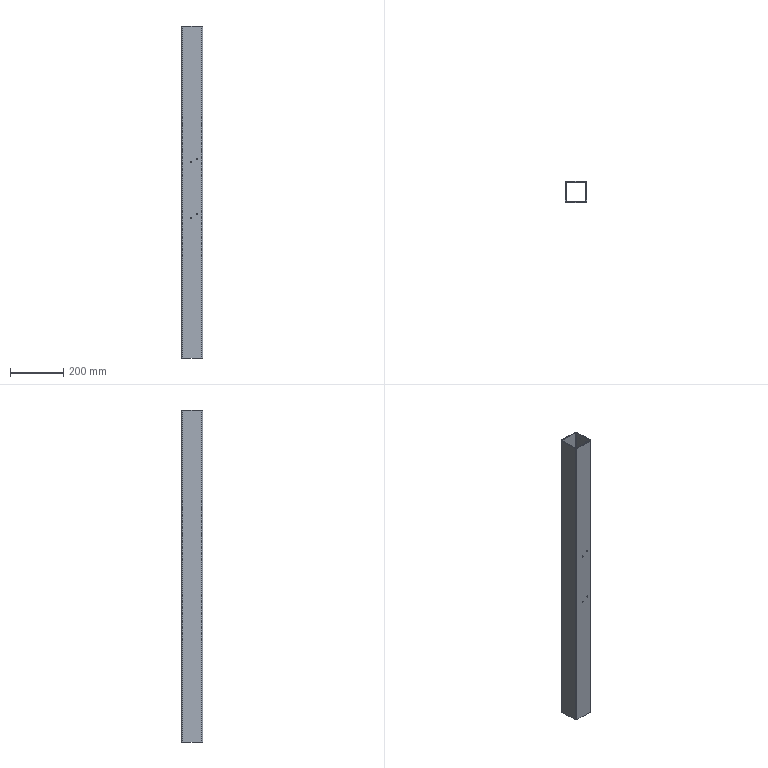Part | SolidWorks | features HoleWzd 3, Extrusion 1, Fillet 1, Shell 1 | 1 solid | 50 faces | box 80 x 80 x 1249 mm | volume 1130618 mm3 | cylinder 40 | plane 10 | commonest cylinder face diameters 5 x32 4 x4 10 x4